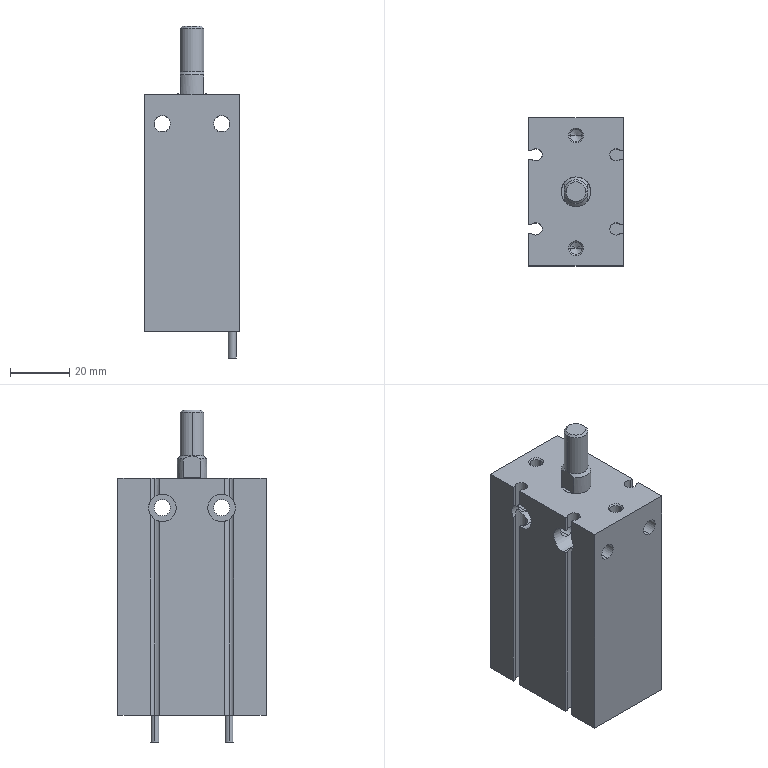Part | STEP file | Bag feed cylinder CDU25-30D-A93L (0) | 1 solid | 139 faces | box 32 x 50 x 112 mm | volume 120089 mm3 | cylinder 60 | plane 51 | cone 28 | commonest cylinder face diameters 5.5 x16 4.134 x12 4.2 x12 9.3 x8 2.7 x4 4 x4